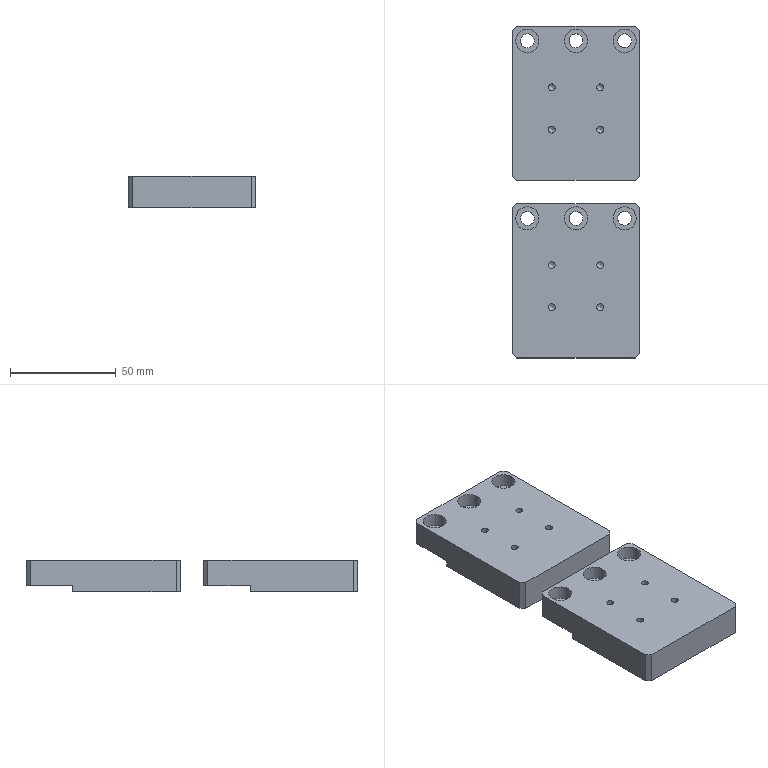Part | 2 solids | 58 faces | box 60 x 157 x 15 mm | volume 117752 mm3 | plane 30 | cylinder 20 | cone 8 | commonest cylinder face diameters 3.3 x8 6.6 x6 11 x6
STEP:
#1=CARTESIAN_POINT('',(-30.,14.5,-7.5));
#2=VERTEX_POINT('',#1);
#3=CARTESIAN_POINT('',(-30.,14.5,-4.5));
#4=VERTEX_POINT('',#3);
#5=CARTESIAN_POINT('',(-30.,14.5,-7.5));
#6=DIRECTION('',(0.,0.,1.));
#7=VECTOR('',#6,1000.);
#8=LINE('',#5,#7);
#9=EDGE_CURVE('',#2,#4,#8,.T.);
#10=ORIENTED_EDGE('',*,*,#9,.T.);
#11=CARTESIAN_POINT('',(30.,14.5,-4.5));
#12=VERTEX_POINT('',#11);
#13=CARTESIAN_POINT('',(30.,14.5,-4.5));
#14=DIRECTION('',(-1.,0.,0.));
#15=VECTOR('',#14,1000.);
#16=LINE('',#13,#15);
#17=EDGE_CURVE('',#12,#4,#16,.T.);
#18=ORIENTED_EDGE('',*,*,#17,.F.);
#19=CARTESIAN_POINT('',(30.,14.5,-7.5));
#20=VERTEX_POINT('',#19);
#21=CARTESIAN_POINT('',(30.,14.5,-7.5));
#22=DIRECTION('',(0.,0.,1.));
#23=VECTOR('',#22,1000.);
#24=LINE('',#21,#23);
#25=EDGE_CURVE('',#20,#12,#24,.T.);
#26=ORIENTED_EDGE('',*,*,#25,.F.);
#27=CARTESIAN_POINT('',(30.,14.5,-7.5));
#28=DIRECTION('',(-1.,0.,0.));
#29=VECTOR('',#28,1000.);
#30=LINE('',#27,#29);
#31=EDGE_CURVE('',#20,#2,#30,.T.);
#32=ORIENTED_EDGE('',*,*,#31,.T.);
#33=EDGE_LOOP('',(#10,#18,#26,#32));
#34=FACE_BOUND('',#33,.T.);
#35=CARTESIAN_POINT('',(30.,14.5,-7.5));
#36=DIRECTION('',(0.,-1.,0.));
#37=DIRECTION('',(1.,0.,0.));
#38=AXIS2_PLACEMENT_3D('',#35,#36,#37);
#39=PLANE('',#38);
#40=ADVANCED_FACE('',(#34),#39,.F.);
#41=CARTESIAN_POINT('',(0.,26.2,-4.5));
#42=VERTEX_POINT('',#41);
#43=CARTESIAN_POINT('',(0.,29.5,-4.5));
#44=DIRECTION('',(0.,0.,-1.));
#45=DIRECTION('',(0.,-1.,0.));
#46=AXIS2_PLACEMENT_3D('',#43,#44,#45);
#47=CIRCLE('',#46,3.3);
#48=EDGE_CURVE('',#42,#42,#47,.T.);
#49=ORIENTED_EDGE('',*,*,#48,.F.);
#50=EDGE_LOOP('',(#49));
#51=FACE_BOUND('',#50,.T.);
#52=CARTESIAN_POINT('',(23.,26.2,-4.5));
#53=VERTEX_POINT('',#52);
#54=CARTESIAN_POINT('',(23.,29.5,-4.5));
#55=DIRECTION('',(0.,0.,-1.));
#56=DIRECTION('',(0.,-1.,0.));
#57=AXIS2_PLACEMENT_3D('',#54,#55,#56);
#58=CIRCLE('',#57,3.3);
#59=EDGE_CURVE('',#53,#53,#58,.T.);
#60=ORIENTED_EDGE('',*,*,#59,.F.);
#61=EDGE_LOOP('',(#60));
#62=FACE_BOUND('',#61,.T.);
#63=CARTESIAN_POINT('',(-23.,26.2,-4.5));
#64=VERTEX_POINT('',#63);
#65=CARTESIAN_POINT('',(-23.,29.5,-4.5));
#66=DIRECTION('',(0.,0.,-1.));
#67=DIRECTION('',(0.,-1.,0.));
#68=AXIS2_PLACEMENT_3D('',#65,#66,#67);
#69=CIRCLE('',#68,3.3);
#70=EDGE_CURVE('',#64,#64,#69,.T.);
#71=ORIENTED_EDGE('',*,*,#70,.F.);
#72=EDGE_LOOP('',(#71));
#73=FACE_BOUND('',#72,.T.);
#74=CARTESIAN_POINT('',(28.,36.5,-4.5));
#75=VERTEX_POINT('',#74);
#76=CARTESIAN_POINT('',(30.,34.5,-4.5));
#77=VERTEX_POINT('',#76);
#78=CARTESIAN_POINT('',(28.,36.5,-4.5));
#79=DIRECTION('',(0.7071,-0.7071,0.));
#80=VECTOR('',#79,1000.);
#81=LINE('',#78,#80);
#82=EDGE_CURVE('',#75,#77,#81,.T.);
#83=ORIENTED_EDGE('',*,*,#82,.T.);
#84=CARTESIAN_POINT('',(30.,36.5,-4.5));
#85=DIRECTION('',(0.,1.,0.));
#86=VECTOR('',#85,1000.);
#87=LINE('',#84,#86);
#88=EDGE_CURVE('',#12,#77,#87,.T.);
#89=ORIENTED_EDGE('',*,*,#88,.F.);
#90=ORIENTED_EDGE('',*,*,#17,.T.);
#91=CARTESIAN_POINT('',(-30.,34.5,-4.5));
#92=VERTEX_POINT('',#91);
#93=CARTESIAN_POINT('',(-30.,36.5,-4.5));
#94=DIRECTION('',(0.,1.,0.));
#95=VECTOR('',#94,1000.);
#96=LINE('',#93,#95);
#97=EDGE_CURVE('',#4,#92,#96,.T.);
#98=ORIENTED_EDGE('',*,*,#97,.T.);
#99=CARTESIAN_POINT('',(-28.,36.5,-4.5));
#100=VERTEX_POINT('',#99);
#101=CARTESIAN_POINT('',(-30.,34.5,-4.5));
#102=DIRECTION('',(0.7071,0.7071,0.));
#103=VECTOR('',#102,1000.);
#104=LINE('',#101,#103);
#105=EDGE_CURVE('',#92,#100,#104,.T.);
#106=ORIENTED_EDGE('',*,*,#105,.T.);
#107=CARTESIAN_POINT('',(30.,36.5,-4.5));
#108=DIRECTION('',(-1.,0.,0.));
#109=VECTOR('',#108,1000.);
#110=LINE('',#107,#109);
#111=EDGE_CURVE('',#75,#100,#110,.T.);
#112=ORIENTED_EDGE('',*,*,#111,.F.);
#113=EDGE_LOOP('',(#83,#89,#90,#98,#106,#112));
#114=FACE_BOUND('',#113,.T.);
#115=CARTESIAN_POINT('',(30.,36.5,-4.5));
#116=DIRECTION('',(0.,0.,1.));
#117=DIRECTION('',(0.,-1.,0.));
#118=AXIS2_PLACEMENT_3D('',#115,#116,#117);
#119=PLANE('',#118);
#120=ADVANCED_FACE('',(#51,#62,#73,#114),#119,.F.);
#121=CARTESIAN_POINT('',(28.5,29.5,1.1));
#122=VERTEX_POINT('',#121);
#123=CARTESIAN_POINT('',(23.,29.5,1.1));
#124=DIRECTION('',(0.,0.,1.));
#125=DIRECTION('',(1.,0.,0.));
#126=AXIS2_PLACEMENT_3D('',#123,#124,#125);
#127=CIRCLE('',#126,5.5);
#128=EDGE_CURVE('',#122,#122,#127,.T.);
#129=ORIENTED_EDGE('',*,*,#128,.T.);
#130=EDGE_LOOP('',(#129));
#131=FACE_BOUND('',#130,.T.);
#132=CARTESIAN_POINT('',(26.3,29.5,1.1));
#133=VERTEX_POINT('',#132);
#134=CARTESIAN_POINT('',(23.,29.5,1.1));
#135=DIRECTION('',(0.,0.,1.));
#136=DIRECTION('',(1.,0.,0.));
#137=AXIS2_PLACEMENT_3D('',#134,#135,#136);
#138=CIRCLE('',#137,3.3);
#139=EDGE_CURVE('',#133,#133,#138,.T.);
#140=ORIENTED_EDGE('',*,*,#139,.F.);
#141=EDGE_LOOP('',(#140));
#142=FACE_BOUND('',#141,.T.);
#143=CARTESIAN_POINT('',(26.3,29.5,1.1));
#144=DIRECTION('',(0.,0.,-1.));
#145=DIRECTION('',(-1.,0.,0.));
#146=AXIS2_PLACEMENT_3D('',#143,#144,#145);
#147=PLANE('',#146);
#148=ADVANCED_FACE('',(#131,#142),#147,.F.);
#149=CARTESIAN_POINT('',(-28.5,29.5,1.1));
#150=VERTEX_POINT('',#149);
#151=CARTESIAN_POINT('',(-23.,29.5,1.1));
#152=DIRECTION('',(0.,0.,1.));
#153=DIRECTION('',(-1.,0.,0.));
#154=AXIS2_PLACEMENT_3D('',#151,#152,#153);
#155=CIRCLE('',#154,5.5);
#156=EDGE_CURVE('',#150,#150,#155,.T.);
#157=ORIENTED_EDGE('',*,*,#156,.T.);
#158=EDGE_LOOP('',(#157));
#159=FACE_BOUND('',#158,.T.);
#160=CARTESIAN_POINT('',(-26.3,29.5,1.1));
#161=VERTEX_POINT('',#160);
#162=CARTESIAN_POINT('',(-23.,29.5,1.1));
#163=DIRECTION('',(0.,0.,1.));
#164=DIRECTION('',(-1.,0.,0.));
#165=AXIS2_PLACEMENT_3D('',#162,#163,#164);
#166=CIRCLE('',#165,3.3);
#167=EDGE_CURVE('',#161,#161,#166,.T.);
#168=ORIENTED_EDGE('',*,*,#167,.F.);
#169=EDGE_LOOP('',(#168));
#170=FACE_BOUND('',#169,.T.);
#171=CARTESIAN_POINT('',(26.3,29.5,1.1));
#172=DIRECTION('',(0.,0.,-1.));
#173=DIRECTION('',(-1.,0.,0.));
#174=AXIS2_PLACEMENT_3D('',#171,#172,#173);
#175=PLANE('',#174);
#176=ADVANCED_FACE('',(#159,#170),#175,.F.);
#177=CARTESIAN_POINT('',(-5.5,29.5,1.1));
#178=VERTEX_POINT('',#177);
#179=CARTESIAN_POINT('',(0.,29.5,1.1));
#180=DIRECTION('',(0.,0.,1.));
#181=DIRECTION('',(-1.,0.,0.));
#182=AXIS2_PLACEMENT_3D('',#179,#180,#181);
#183=CIRCLE('',#182,5.5);
#184=EDGE_CURVE('',#178,#178,#183,.T.);
#185=ORIENTED_EDGE('',*,*,#184,.T.);
#186=EDGE_LOOP('',(#185));
#187=FACE_BOUND('',#186,.T.);
#188=CARTESIAN_POINT('',(-3.3,29.5,1.1));
#189=VERTEX_POINT('',#188);
#190=CARTESIAN_POINT('',(0.,29.5,1.1));
#191=DIRECTION('',(0.,0.,1.));
#192=DIRECTION('',(-1.,0.,0.));
#193=AXIS2_PLACEMENT_3D('',#190,#191,#192);
#194=CIRCLE('',#193,3.3);
#195=EDGE_CURVE('',#189,#189,#194,.T.);
#196=ORIENTED_EDGE('',*,*,#195,.F.);
#197=EDGE_LOOP('',(#196));
#198=FACE_BOUND('',#197,.T.);
#199=CARTESIAN_POINT('',(26.3,29.5,1.1));
#200=DIRECTION('',(0.,0.,-1.));
#201=DIRECTION('',(-1.,0.,0.));
#202=AXIS2_PLACEMENT_3D('',#199,#200,#201);
#203=PLANE('',#202);
#204=ADVANCED_FACE('',(#187,#198),#203,.F.);
#205=ORIENTED_EDGE('',*,*,#105,.F.);
#206=CARTESIAN_POINT('',(-30.,34.5,7.5));
#207=VERTEX_POINT('',#206);
#208=CARTESIAN_POINT('',(-30.,34.5,7.5));
#209=DIRECTION('',(0.,0.,-1.));
#210=VECTOR('',#209,1000.);
#211=LINE('',#208,#210);
#212=EDGE_CURVE('',#207,#92,#211,.T.);
#213=ORIENTED_EDGE('',*,*,#212,.F.);
#214=CARTESIAN_POINT('',(-28.,36.5,7.5));
#215=VERTEX_POINT('',#214);
#216=CARTESIAN_POINT('',(-32.25,32.25,7.5));
#217=DIRECTION('',(-0.7071,-0.7071,0.));
#218=VECTOR('',#217,1000.);
#219=LINE('',#216,#218);
#220=EDGE_CURVE('',#215,#207,#219,.T.);
#221=ORIENTED_EDGE('',*,*,#220,.F.);
#222=CARTESIAN_POINT('',(-28.,36.5,7.5));
#223=DIRECTION('',(0.,0.,1.));
#224=VECTOR('',#223,1000.);
#225=LINE('',#222,#224);
#226=EDGE_CURVE('',#100,#215,#225,.T.);
#227=ORIENTED_EDGE('',*,*,#226,.F.);
#228=EDGE_LOOP('',(#205,#213,#221,#227));
#229=FACE_BOUND('',#228,.T.);
#230=CARTESIAN_POINT('',(-30.,34.5,7.5));
#231=DIRECTION('',(0.7071,-0.7071,0.));
#232=DIRECTION('',(0.,0.,-1.));
#233=AXIS2_PLACEMENT_3D('',#230,#231,#232);
#234=PLANE('',#233);
#235=ADVANCED_FACE('',(#229),#234,.F.);
#236=ORIENTED_EDGE('',*,*,#82,.F.);
#237=CARTESIAN_POINT('',(28.,36.5,7.5));
#238=VERTEX_POINT('',#237);
#239=CARTESIAN_POINT('',(28.,36.5,7.5));
#240=DIRECTION('',(0.,0.,-1.));
#241=VECTOR('',#240,1000.);
#242=LINE('',#239,#241);
#243=EDGE_CURVE('',#238,#75,#242,.T.);
#244=ORIENTED_EDGE('',*,*,#243,.F.);
#245=CARTESIAN_POINT('',(30.,34.5,7.5));
#246=VERTEX_POINT('',#245);
#247=CARTESIAN_POINT('',(32.25,32.25,7.5));
#248=DIRECTION('',(-0.7071,0.7071,0.));
#249=VECTOR('',#248,1000.);
#250=LINE('',#247,#249);
#251=EDGE_CURVE('',#246,#238,#250,.T.);
#252=ORIENTED_EDGE('',*,*,#251,.F.);
#253=CARTESIAN_POINT('',(30.,34.5,7.5));
#254=DIRECTION('',(0.,0.,1.));
#255=VECTOR('',#254,1000.);
#256=LINE('',#253,#255);
#257=EDGE_CURVE('',#77,#246,#256,.T.);
#258=ORIENTED_EDGE('',*,*,#257,.F.);
#259=EDGE_LOOP('',(#236,#244,#252,#258));
#260=FACE_BOUND('',#259,.T.);
#261=CARTESIAN_POINT('',(28.,36.5,7.5));
#262=DIRECTION('',(-0.7071,-0.7071,0.));
#263=DIRECTION('',(0.,0.,-1.));
#264=AXIS2_PLACEMENT_3D('',#261,#262,#263);
#265=PLANE('',#264);
#266=ADVANCED_FACE('',(#260),#265,.F.);
#267=CARTESIAN_POINT('',(28.,-36.5,7.5));
#268=VERTEX_POINT('',#267);
#269=CARTESIAN_POINT('',(30.,-34.5,7.5));
#270=VERTEX_POINT('',#269);
#271=CARTESIAN_POINT('',(32.25,-32.25,7.5));
#272=DIRECTION('',(0.7071,0.7071,0.));
#273=VECTOR('',#272,1000.);
#274=LINE('',#271,#273);
#275=EDGE_CURVE('',#268,#270,#274,.T.);
#276=ORIENTED_EDGE('',*,*,#275,.F.);
#277=CARTESIAN_POINT('',(28.,-36.5,-7.5));
#278=VERTEX_POINT('',#277);
#279=CARTESIAN_POINT('',(28.,-36.5,7.5));
#280=DIRECTION('',(0.,0.,1.));
#281=VECTOR('',#280,1000.);
#282=LINE('',#279,#281);
#283=EDGE_CURVE('',#278,#268,#282,.T.);
#284=ORIENTED_EDGE('',*,*,#283,.F.);
#285=CARTESIAN_POINT('',(30.,-34.5,-7.5));
#286=VERTEX_POINT('',#285);
#287=CARTESIAN_POINT('',(30.,-34.5,-7.5));
#288=DIRECTION('',(-0.7071,-0.7071,0.));
#289=VECTOR('',#288,1000.);
#290=LINE('',#287,#289);
#291=EDGE_CURVE('',#286,#278,#290,.T.);
#292=ORIENTED_EDGE('',*,*,#291,.F.);
#293=CARTESIAN_POINT('',(30.,-34.5,7.5));
#294=DIRECTION('',(0.,0.,-1.));
#295=VECTOR('',#294,1000.);
#296=LINE('',#293,#295);
#297=EDGE_CURVE('',#270,#286,#296,.T.);
#298=ORIENTED_EDGE('',*,*,#297,.F.);
#299=EDGE_LOOP('',(#276,#284,#292,#298));
#300=FACE_BOUND('',#299,.T.);
#301=CARTESIAN_POINT('',(30.,-34.5,7.5));
#302=DIRECTION('',(-0.7071,0.7071,0.));
#303=DIRECTION('',(0.,0.,-1.));
#304=AXIS2_PLACEMENT_3D('',#301,#302,#303);
#305=PLANE('',#304);
#306=ADVANCED_FACE('',(#300),#305,.F.);
#307=CARTESIAN_POINT('',(-30.,-34.5,7.5));
#308=VERTEX_POINT('',#307);
#309=CARTESIAN_POINT('',(-28.,-36.5,7.5));
#310=VERTEX_POINT('',#309);
#311=CARTESIAN_POINT('',(-32.25,-32.25,7.5));
#312=DIRECTION('',(0.7071,-0.7071,0.));
#313=VECTOR('',#312,1000.);
#314=LINE('',#311,#313);
#315=EDGE_CURVE('',#308,#310,#314,.T.);
#316=ORIENTED_EDGE('',*,*,#315,.F.);
#317=CARTESIAN_POINT('',(-30.,-34.5,-7.5));
#318=VERTEX_POINT('',#317);
#319=CARTESIAN_POINT('',(-30.,-34.5,7.5));
#320=DIRECTION('',(0.,0.,1.));
#321=VECTOR('',#320,1000.);
#322=LINE('',#319,#321);
#323=EDGE_CURVE('',#318,#308,#322,.T.);
#324=ORIENTED_EDGE('',*,*,#323,.F.);
#325=CARTESIAN_POINT('',(-28.,-36.5,-7.5));
#326=VERTEX_POINT('',#325);
#327=CARTESIAN_POINT('',(-28.,-36.5,-7.5));
#328=DIRECTION('',(-0.7071,0.7071,0.));
#329=VECTOR('',#328,1000.);
#330=LINE('',#327,#329);
#331=EDGE_CURVE('',#326,#318,#330,.T.);
#332=ORIENTED_EDGE('',*,*,#331,.F.);
#333=CARTESIAN_POINT('',(-28.,-36.5,7.5));
#334=DIRECTION('',(0.,0.,-1.));
#335=VECTOR('',#334,1000.);
#336=LINE('',#333,#335);
#337=EDGE_CURVE('',#310,#326,#336,.T.);
#338=ORIENTED_EDGE('',*,*,#337,.F.);
#339=EDGE_LOOP('',(#316,#324,#332,#338));
#340=FACE_BOUND('',#339,.T.);
#341=CARTESIAN_POINT('',(-28.,-36.5,7.5));
#342=DIRECTION('',(0.7071,0.7071,0.));
#343=DIRECTION('',(0.,0.,-1.));
#344=AXIS2_PLACEMENT_3D('',#341,#342,#343);
#345=PLANE('',#344);
#346=ADVANCED_FACE('',(#340),#345,.F.);
#347=CARTESIAN_POINT('',(-30.,36.5,-7.5));
#348=DIRECTION('',(0.,-1.,0.));
#349=VECTOR('',#348,1000.);
#350=LINE('',#347,#349);
#351=EDGE_CURVE('',#2,#318,#350,.T.);
#352=ORIENTED_EDGE('',*,*,#351,.F.);
#353=ORIENTED_EDGE('',*,*,#31,.F.);
#354=CARTESIAN_POINT('',(30.,36.5,-7.5));
#355=DIRECTION('',(0.,1.,0.));
#356=VECTOR('',#355,1000.);
#357=LINE('',#354,#356);
#358=EDGE_CURVE('',#286,#20,#357,.T.);
#359=ORIENTED_EDGE('',*,*,#358,.F.);
#360=ORIENTED_EDGE('',*,*,#291,.T.);
#361=CARTESIAN_POINT('',(-30.,-36.5,-7.5));
#362=DIRECTION('',(1.,0.,0.));
#363=VECTOR('',#362,1000.);
#364=LINE('',#361,#363);
#365=EDGE_CURVE('',#326,#278,#364,.T.);
#366=ORIENTED_EDGE('',*,*,#365,.F.);
#367=ORIENTED_EDGE('',*,*,#331,.T.);
#368=EDGE_LOOP('',(#352,#353,#359,#360,#366,#367));
#369=FACE_BOUND('',#368,.T.);
#370=CARTESIAN_POINT('',(0.,0.,-7.5));
#371=DIRECTION('',(0.,0.,1.));
#372=DIRECTION('',(1.,0.,0.));
#373=AXIS2_PLACEMENT_3D('',#370,#371,#372);
#374=PLANE('',#373);
#375=ADVANCED_FACE('',(#369),#374,.F.);
#376=CARTESIAN_POINT('',(-30.,36.5,7.5));
#377=DIRECTION('',(0.,-1.,0.));
#378=VECTOR('',#377,1000.);
#379=LINE('',#376,#378);
#380=EDGE_CURVE('',#207,#308,#379,.T.);
#381=ORIENTED_EDGE('',*,*,#380,.T.);
#382=ORIENTED_EDGE('',*,*,#315,.T.);
#383=CARTESIAN_POINT('',(-30.,-36.5,7.5));
#384=DIRECTION('',(1.,0.,0.));
#385=VECTOR('',#384,1000.);
#386=LINE('',#383,#385);
#387=EDGE_CURVE('',#310,#268,#386,.T.);
#388=ORIENTED_EDGE('',*,*,#387,.T.);
#389=ORIENTED_EDGE('',*,*,#275,.T.);
#390=CARTESIAN_POINT('',(30.,36.5,7.5));
#391=DIRECTION('',(0.,1.,0.));
#392=VECTOR('',#391,1000.);
#393=LINE('',#390,#392);
#394=EDGE_CURVE('',#270,#246,#393,.T.);
#395=ORIENTED_EDGE('',*,*,#394,.T.);
#396=ORIENTED_EDGE('',*,*,#251,.T.);
#397=CARTESIAN_POINT('',(-30.,36.5,7.5));
#398=DIRECTION('',(-1.,0.,0.));
#399=VECTOR('',#398,1000.);
#400=LINE('',#397,#399);
#401=EDGE_CURVE('',#238,#215,#400,.T.);
#402=ORIENTED_EDGE('',*,*,#401,.T.);
#403=ORIENTED_EDGE('',*,*,#220,.T.);
#404=EDGE_LOOP('',(#381,#382,#388,#389,#395,#396,#402,#403));
#405=FACE_BOUND('',#404,.T.);
#406=CARTESIAN_POINT('',(13.15,7.5,7.5));
#407=VERTEX_POINT('',#406);
#408=CARTESIAN_POINT('',(11.5,7.5,7.5));
#409=DIRECTION('',(0.,0.,1.));
#410=DIRECTION('',(1.,0.,0.));
#411=AXIS2_PLACEMENT_3D('',#408,#409,#410);
#412=CIRCLE('',#411,1.65);
#413=EDGE_CURVE('',#407,#407,#412,.T.);
#414=ORIENTED_EDGE('',*,*,#413,.F.);
#415=EDGE_LOOP('',(#414));
#416=FACE_BOUND('',#415,.T.);
#417=CARTESIAN_POINT('',(13.15,-12.5,7.5));
#418=VERTEX_POINT('',#417);
#419=CARTESIAN_POINT('',(11.5,-12.5,7.5));
#420=DIRECTION('',(0.,0.,1.));
#421=DIRECTION('',(1.,0.,0.));
#422=AXIS2_PLACEMENT_3D('',#419,#420,#421);
#423=CIRCLE('',#422,1.65);
#424=EDGE_CURVE('',#418,#418,#423,.T.);
#425=ORIENTED_EDGE('',*,*,#424,.F.);
#426=EDGE_LOOP('',(#425));
#427=FACE_BOUND('',#426,.T.);
#428=CARTESIAN_POINT('',(-9.85,-12.5,7.5));
#429=VERTEX_POINT('',#428);
#430=CARTESIAN_POINT('',(-11.5,-12.5,7.5));
#431=DIRECTION('',(0.,0.,1.));
#432=DIRECTION('',(1.,0.,0.));
#433=AXIS2_PLACEMENT_3D('',#430,#431,#432);
#434=CIRCLE('',#433,1.65);
#435=EDGE_CURVE('',#429,#429,#434,.T.);
#436=ORIENTED_EDGE('',*,*,#435,.F.);
#437=EDGE_LOOP('',(#436));
#438=FACE_BOUND('',#437,.T.);
#439=CARTESIAN_POINT('',(-9.85,7.5,7.5));
#440=VERTEX_POINT('',#439);
#441=CARTESIAN_POINT('',(-11.5,7.5,7.5));
#442=DIRECTION('',(0.,0.,1.));
#443=DIRECTION('',(1.,0.,0.));
#444=AXIS2_PLACEMENT_3D('',#441,#442,#443);
#445=CIRCLE('',#444,1.65);
#446=EDGE_CURVE('',#440,#440,#445,.T.);
#447=ORIENTED_EDGE('',*,*,#446,.F.);
#448=EDGE_LOOP('',(#447));
#449=FACE_BOUND('',#448,.T.);
#450=CARTESIAN_POINT('',(5.5,29.5,7.5));
#451=VERTEX_POINT('',#450);
#452=CARTESIAN_POINT('',(0.,29.5,7.5));
#453=DIRECTION('',(0.,0.,1.));
#454=DIRECTION('',(1.,0.,0.));
#455=AXIS2_PLACEMENT_3D('',#452,#453,#454);
#456=CIRCLE('',#455,5.5);
#457=EDGE_CURVE('',#451,#451,#456,.T.);
#458=ORIENTED_EDGE('',*,*,#457,.F.);
#459=EDGE_LOOP('',(#458));
#460=FACE_BOUND('',#459,.T.);
#461=CARTESIAN_POINT('',(-17.5,29.5,7.5));
#462=VERTEX_POINT('',#461);
#463=CARTESIAN_POINT('',(-23.,29.5,7.5));
#464=DIRECTION('',(0.,0.,1.));
#465=DIRECTION('',(1.,0.,0.));
#466=AXIS2_PLACEMENT_3D('',#463,#464,#465);
#467=CIRCLE('',#466,5.5);
#468=EDGE_CURVE('',#462,#462,#467,.T.);
#469=ORIENTED_EDGE('',*,*,#468,.F.);
#470=EDGE_LOOP('',(#469));
#471=FACE_BOUND('',#470,.T.);
#472=CARTESIAN_POINT('',(28.5,29.5,7.5));
#473=VERTEX_POINT('',#472);
#474=CARTESIAN_POINT('',(23.,29.5,7.5));
#475=DIRECTION('',(0.,0.,1.));
#476=DIRECTION('',(1.,0.,0.));
#477=AXIS2_PLACEMENT_3D('',#474,#475,#476);
#478=CIRCLE('',#477,5.5);
#479=EDGE_CURVE('',#473,#473,#478,.T.);
#480=ORIENTED_EDGE('',*,*,#479,.F.);
#481=EDGE_LOOP('',(#480));
#482=FACE_BOUND('',#481,.T.);
#483=CARTESIAN_POINT('',(0.,0.,7.5));
#484=DIRECTION('',(0.,0.,1.));
#485=DIRECTION('',(1.,0.,0.));
#486=AXIS2_PLACEMENT_3D('',#483,#484,#485);
#487=PLANE('',#486);
#488=ADVANCED_FACE('',(#405,#416,#427,#438,#449,#460,#471,#482),#487,.T.);
#489=ORIENTED_EDGE('',*,*,#387,.F.);
#490=ORIENTED_EDGE('',*,*,#337,.T.);
#491=ORIENTED_EDGE('',*,*,#365,.T.);
#492=ORIENTED_EDGE('',*,*,#283,.T.);
#493=EDGE_LOOP('',(#489,#490,#491,#492));
#494=FACE_BOUND('',#493,.T.);
#495=CARTESIAN_POINT('',(-30.,-36.5,7.5));
#496=DIRECTION('',(0.,1.,0.));
#497=DIRECTION('',(0.,0.,1.));
#498=AXIS2_PLACEMENT_3D('',#495,#496,#497);
#499=PLANE('',#498);
#500=ADVANCED_FACE('',(#494),#499,.F.);
#501=ORIENTED_EDGE('',*,*,#212,.T.);
#502=ORIENTED_EDGE('',*,*,#97,.F.);
#503=ORIENTED_EDGE('',*,*,#9,.F.);
#504=ORIENTED_EDGE('',*,*,#351,.T.);
#505=ORIENTED_EDGE('',*,*,#323,.T.);
#506=ORIENTED_EDGE('',*,*,#380,.F.);
#507=EDGE_LOOP('',(#501,#502,#503,#504,#505,#506));
#508=FACE_BOUND('',#507,.T.);
#509=CARTESIAN_POINT('',(-30.,36.5,7.5));
#510=DIRECTION('',(1.,0.,0.));
#511=DIRECTION('',(0.,1.,0.));
#512=AXIS2_PLACEMENT_3D('',#509,#510,#511);
#513=PLANE('',#512);
#514=ADVANCED_FACE('',(#508),#513,.F.);
#515=ORIENTED_EDGE('',*,*,#243,.T.);
#516=ORIENTED_EDGE('',*,*,#111,.T.);
#517=ORIENTED_EDGE('',*,*,#226,.T.);
#518=ORIENTED_EDGE('',*,*,#401,.F.);
#519=EDGE_LOOP('',(#515,#516,#517,#518));
#520=FACE_BOUND('',#519,.T.);
#521=CARTESIAN_POINT('',(-30.,36.5,7.5));
#522=DIRECTION('',(0.,-1.,0.));
#523=DIRECTION('',(0.,0.,-1.));
#524=AXIS2_PLACEMENT_3D('',#521,#522,#523);
#525=PLANE('',#524);
#526=ADVANCED_FACE('',(#520),#525,.F.);
#527=ORIENTED_EDGE('',*,*,#25,.T.);
#528=ORIENTED_EDGE('',*,*,#88,.T.);
#529=ORIENTED_EDGE('',*,*,#257,.T.);
#530=ORIENTED_EDGE('',*,*,#394,.F.);
#531=ORIENTED_EDGE('',*,*,#297,.T.);
#532=ORIENTED_EDGE('',*,*,#358,.T.);
#533=EDGE_LOOP('',(#527,#528,#529,#530,#531,#532));
#534=FACE_BOUND('',#533,.T.);
#535=CARTESIAN_POINT('',(30.,36.5,7.5));
#536=DIRECTION('',(-1.,0.,0.));
#537=DIRECTION('',(0.,-1.,0.));
#538=AXIS2_PLACEMENT_3D('',#535,#536,#537);
#539=PLANE('',#538);
#540=ADVANCED_FACE('',(#534),#539,.F.);
#541=CARTESIAN_POINT('',(13.15,7.5,-2.6));
#542=VERTEX_POINT('',#541);
#543=CARTESIAN_POINT('',(11.5,7.5,-2.6));
#544=DIRECTION('',(0.,0.,1.));
#545=DIRECTION('',(1.,0.,0.));
#546=AXIS2_PLACEMENT_3D('',#543,#544,#545);
#547=CIRCLE('',#546,1.65);
#548=EDGE_CURVE('',#542,#542,#547,.T.);
#549=ORIENTED_EDGE('',*,*,#548,.T.);
#550=EDGE_LOOP('',(#549));
#551=FACE_BOUND('',#550,.T.);
#552=CARTESIAN_POINT('',(11.5,7.5,-3.591));
#553=VERTEX_POINT('',#552);
#554=VERTEX_LOOP('',#553);
#555=FACE_BOUND('',#554,.T.);
#556=CARTESIAN_POINT('',(11.5,7.5,-2.6));
#557=DIRECTION('',(0.,0.,1.));
#558=DIRECTION('',(1.,0.,0.));
#559=AXIS2_PLACEMENT_3D('',#556,#557,#558);
#560=CONICAL_SURFACE('',#559,1.65,1.03);
#561=ADVANCED_FACE('',(#551,#555),#560,.F.);
#562=ORIENTED_EDGE('',*,*,#548,.F.);
#563=EDGE_LOOP('',(#562));
#564=FACE_BOUND('',#563,.T.);
#565=ORIENTED_EDGE('',*,*,#413,.T.);
#566=EDGE_LOOP('',(#565));
#567=FACE_BOUND('',#566,.T.);
#568=CARTESIAN_POINT('',(11.5,7.5,7.5));
#569=DIRECTION('',(0.,0.,1.));
#570=DIRECTION('',(1.,0.,0.));
#571=AXIS2_PLACEMENT_3D('',#568,#569,#570);
#572=CYLINDRICAL_SURFACE('',#571,1.65);
#573=ADVANCED_FACE('',(#564,#567),#572,.F.);
#574=CARTESIAN_POINT('',(13.15,-12.5,-2.6));
#575=VERTEX_POINT('',#574);
#576=CARTESIAN_POINT('',(11.5,-12.5,-2.6));
#577=DIRECTION('',(0.,0.,1.));
#578=DIRECTION('',(1.,0.,0.));
#579=AXIS2_PLACEMENT_3D('',#576,#577,#578);
#580=CIRCLE('',#579,1.65);
#581=EDGE_CURVE('',#575,#575,#580,.T.);
#582=ORIENTED_EDGE('',*,*,#581,.T.);
#583=EDGE_LOOP('',(#582));
#584=FACE_BOUND('',#583,.T.);
#585=CARTESIAN_POINT('',(11.5,-12.5,-3.591));
#586=VERTEX_POINT('',#585);
#587=VERTEX_LOOP('',#586);
#588=FACE_BOUND('',#587,.T.);
#589=CARTESIAN_POINT('',(11.5,-12.5,-2.6));
#590=DIRECTION('',(0.,0.,1.));
#591=DIRECTION('',(1.,0.,0.));
#592=AXIS2_PLACEMENT_3D('',#589,#590,#591);
#593=CONICAL_SURFACE('',#592,1.65,1.03);
#594=ADVANCED_FACE('',(#584,#588),#593,.F.);
#595=ORIENTED_EDGE('',*,*,#581,.F.);
#596=EDGE_LOOP('',(#595));
#597=FACE_BOUND('',#596,.T.);
#598=ORIENTED_EDGE('',*,*,#424,.T.);
#599=EDGE_LOOP('',(#598));
#600=FACE_BOUND('',#599,.T.);
#601=CARTESIAN_POINT('',(11.5,-12.5,7.5));
#602=DIRECTION('',(0.,0.,1.));
#603=DIRECTION('',(1.,0.,0.));
#604=AXIS2_PLACEMENT_3D('',#601,#602,#603);
#605=CYLINDRICAL_SURFACE('',#604,1.65);
#606=ADVANCED_FACE('',(#597,#600),#605,.F.);
#607=CARTESIAN_POINT('',(-9.85,-12.5,-2.6));
#608=VERTEX_POINT('',#607);
#609=CARTESIAN_POINT('',(-11.5,-12.5,-2.6));
#610=DIRECTION('',(0.,0.,1.));
#611=DIRECTION('',(1.,0.,0.));
#612=AXIS2_PLACEMENT_3D('',#609,#610,#611);
#613=CIRCLE('',#612,1.65);
#614=EDGE_CURVE('',#608,#608,#613,.T.);
#615=ORIENTED_EDGE('',*,*,#614,.T.);
#616=EDGE_LOOP('',(#615));
#617=FACE_BOUND('',#616,.T.);
#618=CARTESIAN_POINT('',(-11.5,-12.5,-3.591));
#619=VERTEX_POINT('',#618);
#620=VERTEX_LOOP('',#619);
#621=FACE_BOUND('',#620,.T.);
#622=CARTESIAN_POINT('',(-11.5,-12.5,-2.6));
#623=DIRECTION('',(0.,0.,1.));
#624=DIRECTION('',(1.,0.,0.));
#625=AXIS2_PLACEMENT_3D('',#622,#623,#624);
#626=CONICAL_SURFACE('',#625,1.65,1.03);
#627=ADVANCED_FACE('',(#617,#621),#626,.F.);
#628=ORIENTED_EDGE('',*,*,#614,.F.);
#629=EDGE_LOOP('',(#628));
#630=FACE_BOUND('',#629,.T.);
#631=ORIENTED_EDGE('',*,*,#435,.T.);
#632=EDGE_LOOP('',(#631));
#633=FACE_BOUND('',#632,.T.);
#634=CARTESIAN_POINT('',(-11.5,-12.5,7.5));
#635=DIRECTION('',(0.,0.,1.));
#636=DIRECTION('',(1.,0.,0.));
#637=AXIS2_PLACEMENT_3D('',#634,#635,#636);
#638=CYLINDRICAL_SURFACE('',#637,1.65);
#639=ADVANCED_FACE('',(#630,#633),#638,.F.);
#640=CARTESIAN_POINT('',(-9.85,7.5,-2.6));
#641=VERTEX_POINT('',#640);
#642=CARTESIAN_POINT('',(-11.5,7.5,-2.6));
#643=DIRECTION('',(0.,0.,1.));
#644=DIRECTION('',(1.,0.,0.));
#645=AXIS2_PLACEMENT_3D('',#642,#643,#644);
#646=CIRCLE('',#645,1.65);
#647=EDGE_CURVE('',#641,#641,#646,.T.);
#648=ORIENTED_EDGE('',*,*,#647,.T.);
#649=EDGE_LOOP('',(#648));
#650=FACE_BOUND('',#649,.T.);
#651=CARTESIAN_POINT('',(-11.5,7.5,-3.591));
#652=VERTEX_POINT('',#651);
#653=VERTEX_LOOP('',#652);
#654=FACE_BOUND('',#653,.T.);
#655=CARTESIAN_POINT('',(-11.5,7.5,-2.6));
#656=DIRECTION('',(0.,0.,1.));
#657=DIRECTION('',(1.,0.,0.));
#658=AXIS2_PLACEMENT_3D('',#655,#656,#657);
#659=CONICAL_SURFACE('',#658,1.65,1.03);
#660=ADVANCED_FACE('',(#650,#654),#659,.F.);
#661=ORIENTED_EDGE('',*,*,#647,.F.);
#662=EDGE_LOOP('',(#661));
#663=FACE_BOUND('',#662,.T.);
#664=ORIENTED_EDGE('',*,*,#446,.T.);
#665=EDGE_LOOP('',(#664));
#666=FACE_BOUND('',#665,.T.);
#667=CARTESIAN_POINT('',(-11.5,7.5,7.5));
#668=DIRECTION('',(0.,0.,1.));
#669=DIRECTION('',(1.,0.,0.));
#670=AXIS2_PLACEMENT_3D('',#667,#668,#669);
#671=CYLINDRICAL_SURFACE('',#670,1.65);
#672=ADVANCED_FACE('',(#663,#666),#671,.F.);
#673=ORIENTED_EDGE('',*,*,#48,.T.);
#674=EDGE_LOOP('',(#673));
#675=FACE_BOUND('',#674,.T.);
#676=ORIENTED_EDGE('',*,*,#195,.T.);
#677=EDGE_LOOP('',(#676));
#678=FACE_BOUND('',#677,.T.);
#679=CARTESIAN_POINT('',(0.,29.5,7.5));
#680=DIRECTION('',(0.,0.,1.));
#681=DIRECTION('',(1.,0.,0.));
#682=AXIS2_PLACEMENT_3D('',#679,#680,#681);
#683=CYLINDRICAL_SURFACE('',#682,3.3);
#684=ADVANCED_FACE('',(#675,#678),#683,.F.);
#685=ORIENTED_EDGE('',*,*,#184,.F.);
#686=EDGE_LOOP('',(#685));
#687=FACE_BOUND('',#686,.T.);
#688=ORIENTED_EDGE('',*,*,#457,.T.);
#689=EDGE_LOOP('',(#688));
#690=FACE_BOUND('',#689,.T.);
#691=CARTESIAN_POINT('',(0.,29.5,7.5));
#692=DIRECTION('',(0.,0.,1.));
#693=DIRECTION('',(1.,0.,0.));
#694=AXIS2_PLACEMENT_3D('',#691,#692,#693);
#695=CYLINDRICAL_SURFACE('',#694,5.5);
#696=ADVANCED_FACE('',(#687,#690),#695,.F.);
#697=ORIENTED_EDGE('',*,*,#70,.T.);
#698=EDGE_LOOP('',(#697));
#699=FACE_BOUND('',#698,.T.);
#700=ORIENTED_EDGE('',*,*,#167,.T.);
#701=EDGE_LOOP('',(#700));
#702=FACE_BOUND('',#701,.T.);
#703=CARTESIAN_POINT('',(-23.,29.5,7.5));
#704=DIRECTION('',(0.,0.,1.));
#705=DIRECTION('',(1.,0.,0.));
#706=AXIS2_PLACEMENT_3D('',#703,#704,#705);
#707=CYLINDRICAL_SURFACE('',#706,3.3);
#708=ADVANCED_FACE('',(#699,#702),#707,.F.);
#709=ORIENTED_EDGE('',*,*,#156,.F.);
#710=EDGE_LOOP('',(#709));
#711=FACE_BOUND('',#710,.T.);
#712=ORIENTED_EDGE('',*,*,#468,.T.);
#713=EDGE_LOOP('',(#712));
#714=FACE_BOUND('',#713,.T.);
#715=CARTESIAN_POINT('',(-23.,29.5,7.5));
#716=DIRECTION('',(0.,0.,1.));
#717=DIRECTION('',(1.,0.,0.));
#718=AXIS2_PLACEMENT_3D('',#715,#716,#717);
#719=CYLINDRICAL_SURFACE('',#718,5.5);
#720=ADVANCED_FACE('',(#711,#714),#719,.F.);
#721=ORIENTED_EDGE('',*,*,#59,.T.);
#722=EDGE_LOOP('',(#721));
#723=FACE_BOUND('',#722,.T.);
#724=ORIENTED_EDGE('',*,*,#139,.T.);
#725=EDGE_LOOP('',(#724));
#726=FACE_BOUND('',#725,.T.);
#727=CARTESIAN_POINT('',(23.,29.5,7.5));
#728=DIRECTION('',(0.,0.,1.));
#729=DIRECTION('',(1.,0.,0.));
#730=AXIS2_PLACEMENT_3D('',#727,#728,#729);
#731=CYLINDRICAL_SURFACE('',#730,3.3);
#732=ADVANCED_FACE('',(#723,#726),#731,.F.);
#733=ORIENTED_EDGE('',*,*,#128,.F.);
#734=EDGE_LOOP('',(#733));
#735=FACE_BOUND('',#734,.T.);
#736=ORIENTED_EDGE('',*,*,#479,.T.);
#737=EDGE_LOOP('',(#736));
#738=FACE_BOUND('',#737,.T.);
#739=CARTESIAN_POINT('',(23.,29.5,7.5));
#740=DIRECTION('',(0.,0.,1.));
#741=DIRECTION('',(1.,0.,0.));
#742=AXIS2_PLACEMENT_3D('',#739,#740,#741);
#743=CYLINDRICAL_SURFACE('',#742,5.5);
#744=ADVANCED_FACE('',(#735,#738),#743,.F.);
#745=CLOSED_SHELL('',(#40,#120,#148,#176,#204,#235,#266,#306,#346,#375,#488,#500,#514,#526,#540,#561,#573,#594,#606,#627,#639,#660,#672,#684,#696,#708,#720,#732,#744));
#746=MANIFOLD_SOLID_BREP('',#745);
#747=CARTESIAN_POINT('',(-30.,98.5,-7.5));
#748=VERTEX_POINT('',#747);
#749=CARTESIAN_POINT('',(-30.,98.5,-4.5));
#750=VERTEX_POINT('',#749);
#751=CARTESIAN_POINT('',(-30.,98.5,-7.5));
#752=DIRECTION('',(0.,0.,1.));
#753=VECTOR('',#752,1000.);
#754=LINE('',#751,#753);
#755=EDGE_CURVE('',#748,#750,#754,.T.);
#756=ORIENTED_EDGE('',*,*,#755,.T.);
#757=CARTESIAN_POINT('',(30.,98.5,-4.5));
#758=VERTEX_POINT('',#757);
#759=CARTESIAN_POINT('',(30.,98.5,-4.5));
#760=DIRECTION('',(-1.,0.,0.));
#761=VECTOR('',#760,1000.);
#762=LINE('',#759,#761);
#763=EDGE_CURVE('',#758,#750,#762,.T.);
#764=ORIENTED_EDGE('',*,*,#763,.F.);
#765=CARTESIAN_POINT('',(30.,98.5,-7.5));
#766=VERTEX_POINT('',#765);
#767=CARTESIAN_POINT('',(30.,98.5,-7.5));
#768=DIRECTION('',(0.,0.,1.));
#769=VECTOR('',#768,1000.);
#770=LINE('',#767,#769);
#771=EDGE_CURVE('',#766,#758,#770,.T.);
#772=ORIENTED_EDGE('',*,*,#771,.F.);
#773=CARTESIAN_POINT('',(30.,98.5,-7.5));
#774=DIRECTION('',(-1.,0.,0.));
#775=VECTOR('',#774,1000.);
#776=LINE('',#773,#775);
#777=EDGE_CURVE('',#766,#748,#776,.T.);
#778=ORIENTED_EDGE('',*,*,#777,.T.);
#779=EDGE_LOOP('',(#756,#764,#772,#778));
#780=FACE_BOUND('',#779,.T.);
#781=CARTESIAN_POINT('',(30.,98.5,-7.5));
#782=DIRECTION('',(0.,-1.,0.));
#783=DIRECTION('',(1.,0.,0.));
#784=AXIS2_PLACEMENT_3D('',#781,#782,#783);
#785=PLANE('',#784);
#786=ADVANCED_FACE('',(#780),#785,.F.);
#787=CARTESIAN_POINT('',(0.,110.2,-4.5));
#788=VERTEX_POINT('',#787);
#789=CARTESIAN_POINT('',(0.,113.5,-4.5));
#790=DIRECTION('',(0.,0.,-1.));
#791=DIRECTION('',(0.,-1.,0.));
#792=AXIS2_PLACEMENT_3D('',#789,#790,#791);
#793=CIRCLE('',#792,3.3);
#794=EDGE_CURVE('',#788,#788,#793,.T.);
#795=ORIENTED_EDGE('',*,*,#794,.F.);
#796=EDGE_LOOP('',(#795));
#797=FACE_BOUND('',#796,.T.);
#798=CARTESIAN_POINT('',(23.,110.2,-4.5));
#799=VERTEX_POINT('',#798);
#800=CARTESIAN_POINT('',(23.,113.5,-4.5));
#801=DIRECTION('',(0.,0.,-1.));
#802=DIRECTION('',(0.,-1.,0.));
#803=AXIS2_PLACEMENT_3D('',#800,#801,#802);
#804=CIRCLE('',#803,3.3);
#805=EDGE_CURVE('',#799,#799,#804,.T.);
#806=ORIENTED_EDGE('',*,*,#805,.F.);
#807=EDGE_LOOP('',(#806));
#808=FACE_BOUND('',#807,.T.);
#809=CARTESIAN_POINT('',(-23.,110.2,-4.5));
#810=VERTEX_POINT('',#809);
#811=CARTESIAN_POINT('',(-23.,113.5,-4.5));
#812=DIRECTION('',(0.,0.,-1.));
#813=DIRECTION('',(0.,-1.,0.));
#814=AXIS2_PLACEMENT_3D('',#811,#812,#813);
#815=CIRCLE('',#814,3.3);
#816=EDGE_CURVE('',#810,#810,#815,.T.);
#817=ORIENTED_EDGE('',*,*,#816,.F.);
#818=EDGE_LOOP('',(#817));
#819=FACE_BOUND('',#818,.T.);
#820=CARTESIAN_POINT('',(28.,120.5,-4.5));
#821=VERTEX_POINT('',#820);
#822=CARTESIAN_POINT('',(30.,118.5,-4.5));
#823=VERTEX_POINT('',#822);
#824=CARTESIAN_POINT('',(28.,120.5,-4.5));
#825=DIRECTION('',(0.7071,-0.7071,0.));
#826=VECTOR('',#825,1000.);
#827=LINE('',#824,#826);
#828=EDGE_CURVE('',#821,#823,#827,.T.);
#829=ORIENTED_EDGE('',*,*,#828,.T.);
#830=CARTESIAN_POINT('',(30.,120.5,-4.5));
#831=DIRECTION('',(0.,1.,0.));
#832=VECTOR('',#831,1000.);
#833=LINE('',#830,#832);
#834=EDGE_CURVE('',#758,#823,#833,.T.);
#835=ORIENTED_EDGE('',*,*,#834,.F.);
#836=ORIENTED_EDGE('',*,*,#763,.T.);
#837=CARTESIAN_POINT('',(-30.,118.5,-4.5));
#838=VERTEX_POINT('',#837);
#839=CARTESIAN_POINT('',(-30.,120.5,-4.5));
#840=DIRECTION('',(0.,1.,0.));
#841=VECTOR('',#840,1000.);
#842=LINE('',#839,#841);
#843=EDGE_CURVE('',#750,#838,#842,.T.);
#844=ORIENTED_EDGE('',*,*,#843,.T.);
#845=CARTESIAN_POINT('',(-28.,120.5,-4.5));
#846=VERTEX_POINT('',#845);
#847=CARTESIAN_POINT('',(-30.,118.5,-4.5));
#848=DIRECTION('',(0.7071,0.7071,0.));
#849=VECTOR('',#848,1000.);
#850=LINE('',#847,#849);
#851=EDGE_CURVE('',#838,#846,#850,.T.);
#852=ORIENTED_EDGE('',*,*,#851,.T.);
#853=CARTESIAN_POINT('',(30.,120.5,-4.5));
#854=DIRECTION('',(-1.,0.,0.));
#855=VECTOR('',#854,1000.);
#856=LINE('',#853,#855);
#857=EDGE_CURVE('',#821,#846,#856,.T.);
#858=ORIENTED_EDGE('',*,*,#857,.F.);
#859=EDGE_LOOP('',(#829,#835,#836,#844,#852,#858));
#860=FACE_BOUND('',#859,.T.);
#861=CARTESIAN_POINT('',(30.,120.5,-4.5));
#862=DIRECTION('',(0.,0.,1.));
#863=DIRECTION('',(0.,-1.,0.));
#864=AXIS2_PLACEMENT_3D('',#861,#862,#863);
#865=PLANE('',#864);
#866=ADVANCED_FACE('',(#797,#808,#819,#860),#865,.F.);
#867=CARTESIAN_POINT('',(28.5,113.5,1.1));
#868=VERTEX_POINT('',#867);
#869=CARTESIAN_POINT('',(23.,113.5,1.1));
#870=DIRECTION('',(0.,0.,1.));
#871=DIRECTION('',(1.,0.,0.));
#872=AXIS2_PLACEMENT_3D('',#869,#870,#871);
#873=CIRCLE('',#872,5.5);
#874=EDGE_CURVE('',#868,#868,#873,.T.);
#875=ORIENTED_EDGE('',*,*,#874,.T.);
#876=EDGE_LOOP('',(#875));
#877=FACE_BOUND('',#876,.T.);
#878=CARTESIAN_POINT('',(26.3,113.5,1.1));
#879=VERTEX_POINT('',#878);
#880=CARTESIAN_POINT('',(23.,113.5,1.1));
#881=DIRECTION('',(0.,0.,1.));
#882=DIRECTION('',(1.,0.,0.));
#883=AXIS2_PLACEMENT_3D('',#880,#881,#882);
#884=CIRCLE('',#883,3.3);
#885=EDGE_CURVE('',#879,#879,#884,.T.);
#886=ORIENTED_EDGE('',*,*,#885,.F.);
#887=EDGE_LOOP('',(#886));
#888=FACE_BOUND('',#887,.T.);
#889=CARTESIAN_POINT('',(26.3,113.5,1.1));
#890=DIRECTION('',(0.,0.,-1.));
#891=DIRECTION('',(-1.,0.,0.));
#892=AXIS2_PLACEMENT_3D('',#889,#890,#891);
#893=PLANE('',#892);
#894=ADVANCED_FACE('',(#877,#888),#893,.F.);
#895=CARTESIAN_POINT('',(-28.5,113.5,1.1));
#896=VERTEX_POINT('',#895);
#897=CARTESIAN_POINT('',(-23.,113.5,1.1));
#898=DIRECTION('',(0.,0.,1.));
#899=DIRECTION('',(-1.,0.,0.));
#900=AXIS2_PLACEMENT_3D('',#897,#898,#899);
#901=CIRCLE('',#900,5.5);
#902=EDGE_CURVE('',#896,#896,#901,.T.);
#903=ORIENTED_EDGE('',*,*,#902,.T.);
#904=EDGE_LOOP('',(#903));
#905=FACE_BOUND('',#904,.T.);
#906=CARTESIAN_POINT('',(-26.3,113.5,1.1));
#907=VERTEX_POINT('',#906);
#908=CARTESIAN_POINT('',(-23.,113.5,1.1));
#909=DIRECTION('',(0.,0.,1.));
#910=DIRECTION('',(-1.,0.,0.));
#911=AXIS2_PLACEMENT_3D('',#908,#909,#910);
#912=CIRCLE('',#911,3.3);
#913=EDGE_CURVE('',#907,#907,#912,.T.);
#914=ORIENTED_EDGE('',*,*,#913,.F.);
#915=EDGE_LOOP('',(#914));
#916=FACE_BOUND('',#915,.T.);
#917=CARTESIAN_POINT('',(26.3,113.5,1.1));
#918=DIRECTION('',(0.,0.,-1.));
#919=DIRECTION('',(-1.,0.,0.));
#920=AXIS2_PLACEMENT_3D('',#917,#918,#919);
#921=PLANE('',#920);
#922=ADVANCED_FACE('',(#905,#916),#921,.F.);
#923=CARTESIAN_POINT('',(-5.5,113.5,1.1));
#924=VERTEX_POINT('',#923);
#925=CARTESIAN_POINT('',(0.,113.5,1.1));
#926=DIRECTION('',(0.,0.,1.));
#927=DIRECTION('',(-1.,0.,0.));
#928=AXIS2_PLACEMENT_3D('',#925,#926,#927);
#929=CIRCLE('',#928,5.5);
#930=EDGE_CURVE('',#924,#924,#929,.T.);
#931=ORIENTED_EDGE('',*,*,#930,.T.);
#932=EDGE_LOOP('',(#931));
#933=FACE_BOUND('',#932,.T.);
#934=CARTESIAN_POINT('',(-3.3,113.5,1.1));
#935=VERTEX_POINT('',#934);
#936=CARTESIAN_POINT('',(0.,113.5,1.1));
#937=DIRECTION('',(0.,0.,1.));
#938=DIRECTION('',(-1.,0.,0.));
#939=AXIS2_PLACEMENT_3D('',#936,#937,#938);
#940=CIRCLE('',#939,3.3);
#941=EDGE_CURVE('',#935,#935,#940,.T.);
#942=ORIENTED_EDGE('',*,*,#941,.F.);
#943=EDGE_LOOP('',(#942));
#944=FACE_BOUND('',#943,.T.);
#945=CARTESIAN_POINT('',(26.3,113.5,1.1));
#946=DIRECTION('',(0.,0.,-1.));
#947=DIRECTION('',(-1.,0.,0.));
#948=AXIS2_PLACEMENT_3D('',#945,#946,#947);
#949=PLANE('',#948);
#950=ADVANCED_FACE('',(#933,#944),#949,.F.);
#951=ORIENTED_EDGE('',*,*,#851,.F.);
#952=CARTESIAN_POINT('',(-30.,118.5,7.5));
#953=VERTEX_POINT('',#952);
#954=CARTESIAN_POINT('',(-30.,118.5,7.5));
#955=DIRECTION('',(0.,0.,-1.));
#956=VECTOR('',#955,1000.);
#957=LINE('',#954,#956);
#958=EDGE_CURVE('',#953,#838,#957,.T.);
#959=ORIENTED_EDGE('',*,*,#958,.F.);
#960=CARTESIAN_POINT('',(-28.,120.5,7.5));
#961=VERTEX_POINT('',#960);
#962=CARTESIAN_POINT('',(-32.25,116.25,7.5));
#963=DIRECTION('',(-0.7071,-0.7071,0.));
#964=VECTOR('',#963,1000.);
#965=LINE('',#962,#964);
#966=EDGE_CURVE('',#961,#953,#965,.T.);
#967=ORIENTED_EDGE('',*,*,#966,.F.);
#968=CARTESIAN_POINT('',(-28.,120.5,7.5));
#969=DIRECTION('',(0.,0.,1.));
#970=VECTOR('',#969,1000.);
#971=LINE('',#968,#970);
#972=EDGE_CURVE('',#846,#961,#971,.T.);
#973=ORIENTED_EDGE('',*,*,#972,.F.);
#974=EDGE_LOOP('',(#951,#959,#967,#973));
#975=FACE_BOUND('',#974,.T.);
#976=CARTESIAN_POINT('',(-30.,118.5,7.5));
#977=DIRECTION('',(0.7071,-0.7071,0.));
#978=DIRECTION('',(0.,0.,-1.));
#979=AXIS2_PLACEMENT_3D('',#976,#977,#978);
#980=PLANE('',#979);
#981=ADVANCED_FACE('',(#975),#980,.F.);
#982=ORIENTED_EDGE('',*,*,#828,.F.);
#983=CARTESIAN_POINT('',(28.,120.5,7.5));
#984=VERTEX_POINT('',#983);
#985=CARTESIAN_POINT('',(28.,120.5,7.5));
#986=DIRECTION('',(0.,0.,-1.));
#987=VECTOR('',#986,1000.);
#988=LINE('',#985,#987);
#989=EDGE_CURVE('',#984,#821,#988,.T.);
#990=ORIENTED_EDGE('',*,*,#989,.F.);
#991=CARTESIAN_POINT('',(30.,118.5,7.5));
#992=VERTEX_POINT('',#991);
#993=CARTESIAN_POINT('',(32.25,116.25,7.5));
#994=DIRECTION('',(-0.7071,0.7071,0.));
#995=VECTOR('',#994,1000.);
#996=LINE('',#993,#995);
#997=EDGE_CURVE('',#992,#984,#996,.T.);
#998=ORIENTED_EDGE('',*,*,#997,.F.);
#999=CARTESIAN_POINT('',(30.,118.5,7.5));
#1000=DIRECTION('',(0.,0.,1.));
#1001=VECTOR('',#1000,1000.);
#1002=LINE('',#999,#1001);
#1003=EDGE_CURVE('',#823,#992,#1002,.T.);
#1004=ORIENTED_EDGE('',*,*,#1003,.F.);
#1005=EDGE_LOOP('',(#982,#990,#998,#1004));
#1006=FACE_BOUND('',#1005,.T.);
#1007=CARTESIAN_POINT('',(28.,120.5,7.5));
#1008=DIRECTION('',(-0.7071,-0.7071,0.));
#1009=DIRECTION('',(0.,0.,-1.));
#1010=AXIS2_PLACEMENT_3D('',#1007,#1008,#1009);
#1011=PLANE('',#1010);
#1012=ADVANCED_FACE('',(#1006),#1011,.F.);
#1013=CARTESIAN_POINT('',(28.,47.5,7.5));
#1014=VERTEX_POINT('',#1013);
#1015=CARTESIAN_POINT('',(30.,49.5,7.5));
#1016=VERTEX_POINT('',#1015);
#1017=CARTESIAN_POINT('',(32.25,51.75,7.5));
#1018=DIRECTION('',(0.7071,0.7071,0.));
#1019=VECTOR('',#1018,1000.);
#1020=LINE('',#1017,#1019);
#1021=EDGE_CURVE('',#1014,#1016,#1020,.T.);
#1022=ORIENTED_EDGE('',*,*,#1021,.F.);
#1023=CARTESIAN_POINT('',(28.,47.5,-7.5));
#1024=VERTEX_POINT('',#1023);
#1025=CARTESIAN_POINT('',(28.,47.5,7.5));
#1026=DIRECTION('',(0.,0.,1.));
#1027=VECTOR('',#1026,1000.);
#1028=LINE('',#1025,#1027);
#1029=EDGE_CURVE('',#1024,#1014,#1028,.T.);
#1030=ORIENTED_EDGE('',*,*,#1029,.F.);
#1031=CARTESIAN_POINT('',(30.,49.5,-7.5));
#1032=VERTEX_POINT('',#1031);
#1033=CARTESIAN_POINT('',(30.,49.5,-7.5));
#1034=DIRECTION('',(-0.7071,-0.7071,0.));
#1035=VECTOR('',#1034,1000.);
#1036=LINE('',#1033,#1035);
#1037=EDGE_CURVE('',#1032,#1024,#1036,.T.);
#1038=ORIENTED_EDGE('',*,*,#1037,.F.);
#1039=CARTESIAN_POINT('',(30.,49.5,7.5));
#1040=DIRECTION('',(0.,0.,-1.));
#1041=VECTOR('',#1040,1000.);
#1042=LINE('',#1039,#1041);
#1043=EDGE_CURVE('',#1016,#1032,#1042,.T.);
#1044=ORIENTED_EDGE('',*,*,#1043,.F.);
#1045=EDGE_LOOP('',(#1022,#1030,#1038,#1044));
#1046=FACE_BOUND('',#1045,.T.);
#1047=CARTESIAN_POINT('',(30.,49.5,7.5));
#1048=DIRECTION('',(-0.7071,0.7071,0.));
#1049=DIRECTION('',(0.,0.,-1.));
#1050=AXIS2_PLACEMENT_3D('',#1047,#1048,#1049);
#1051=PLANE('',#1050);
#1052=ADVANCED_FACE('',(#1046),#1051,.F.);
#1053=CARTESIAN_POINT('',(-30.,49.5,7.5));
#1054=VERTEX_POINT('',#1053);
#1055=CARTESIAN_POINT('',(-28.,47.5,7.5));
#1056=VERTEX_POINT('',#1055);
#1057=CARTESIAN_POINT('',(-32.25,51.75,7.5));
#1058=DIRECTION('',(0.7071,-0.7071,0.));
#1059=VECTOR('',#1058,1000.);
#1060=LINE('',#1057,#1059);
#1061=EDGE_CURVE('',#1054,#1056,#1060,.T.);
#1062=ORIENTED_EDGE('',*,*,#1061,.F.);
#1063=CARTESIAN_POINT('',(-30.,49.5,-7.5));
#1064=VERTEX_POINT('',#1063);
#1065=CARTESIAN_POINT('',(-30.,49.5,7.5));
#1066=DIRECTION('',(0.,0.,1.));
#1067=VECTOR('',#1066,1000.);
#1068=LINE('',#1065,#1067);
#1069=EDGE_CURVE('',#1064,#1054,#1068,.T.);
#1070=ORIENTED_EDGE('',*,*,#1069,.F.);
#1071=CARTESIAN_POINT('',(-28.,47.5,-7.5));
#1072=VERTEX_POINT('',#1071);
#1073=CARTESIAN_POINT('',(-28.,47.5,-7.5));
#1074=DIRECTION('',(-0.7071,0.7071,0.));
#1075=VECTOR('',#1074,1000.);
#1076=LINE('',#1073,#1075);
#1077=EDGE_CURVE('',#1072,#1064,#1076,.T.);
#1078=ORIENTED_EDGE('',*,*,#1077,.F.);
#1079=CARTESIAN_POINT('',(-28.,47.5,7.5));
#1080=DIRECTION('',(0.,0.,-1.));
#1081=VECTOR('',#1080,1000.);
#1082=LINE('',#1079,#1081);
#1083=EDGE_CURVE('',#1056,#1072,#1082,.T.);
#1084=ORIENTED_EDGE('',*,*,#1083,.F.);
#1085=EDGE_LOOP('',(#1062,#1070,#1078,#1084));
#1086=FACE_BOUND('',#1085,.T.);
#1087=CARTESIAN_POINT('',(-28.,47.5,7.5));
#1088=DIRECTION('',(0.7071,0.7071,0.));
#1089=DIRECTION('',(0.,0.,-1.));
#1090=AXIS2_PLACEMENT_3D('',#1087,#1088,#1089);
#1091=PLANE('',#1090);
#1092=ADVANCED_FACE('',(#1086),#1091,.F.);
#1093=CARTESIAN_POINT('',(-30.,120.5,-7.5));
#1094=DIRECTION('',(0.,-1.,0.));
#1095=VECTOR('',#1094,1000.);
#1096=LINE('',#1093,#1095);
#1097=EDGE_CURVE('',#748,#1064,#1096,.T.);
#1098=ORIENTED_EDGE('',*,*,#1097,.F.);
#1099=ORIENTED_EDGE('',*,*,#777,.F.);
#1100=CARTESIAN_POINT('',(30.,120.5,-7.5));
#1101=DIRECTION('',(0.,1.,0.));
#1102=VECTOR('',#1101,1000.);
#1103=LINE('',#1100,#1102);
#1104=EDGE_CURVE('',#1032,#766,#1103,.T.);
#1105=ORIENTED_EDGE('',*,*,#1104,.F.);
#1106=ORIENTED_EDGE('',*,*,#1037,.T.);
#1107=CARTESIAN_POINT('',(-30.,47.5,-7.5));
#1108=DIRECTION('',(1.,0.,0.));
#1109=VECTOR('',#1108,1000.);
#1110=LINE('',#1107,#1109);
#1111=EDGE_CURVE('',#1072,#1024,#1110,.T.);
#1112=ORIENTED_EDGE('',*,*,#1111,.F.);
#1113=ORIENTED_EDGE('',*,*,#1077,.T.);
#1114=EDGE_LOOP('',(#1098,#1099,#1105,#1106,#1112,#1113));
#1115=FACE_BOUND('',#1114,.T.);
#1116=CARTESIAN_POINT('',(0.,84.,-7.5));
#1117=DIRECTION('',(0.,0.,1.));
#1118=DIRECTION('',(1.,0.,0.));
#1119=AXIS2_PLACEMENT_3D('',#1116,#1117,#1118);
#1120=PLANE('',#1119);
#1121=ADVANCED_FACE('',(#1115),#1120,.F.);
#1122=CARTESIAN_POINT('',(-30.,120.5,7.5));
#1123=DIRECTION('',(0.,-1.,0.));
#1124=VECTOR('',#1123,1000.);
#1125=LINE('',#1122,#1124);
#1126=EDGE_CURVE('',#953,#1054,#1125,.T.);
#1127=ORIENTED_EDGE('',*,*,#1126,.T.);
#1128=ORIENTED_EDGE('',*,*,#1061,.T.);
#1129=CARTESIAN_POINT('',(-30.,47.5,7.5));
#1130=DIRECTION('',(1.,0.,0.));
#1131=VECTOR('',#1130,1000.);
#1132=LINE('',#1129,#1131);
#1133=EDGE_CURVE('',#1056,#1014,#1132,.T.);
#1134=ORIENTED_EDGE('',*,*,#1133,.T.);
#1135=ORIENTED_EDGE('',*,*,#1021,.T.);
#1136=CARTESIAN_POINT('',(30.,120.5,7.5));
#1137=DIRECTION('',(0.,1.,0.));
#1138=VECTOR('',#1137,1000.);
#1139=LINE('',#1136,#1138);
#1140=EDGE_CURVE('',#1016,#992,#1139,.T.);
#1141=ORIENTED_EDGE('',*,*,#1140,.T.);
#1142=ORIENTED_EDGE('',*,*,#997,.T.);
#1143=CARTESIAN_POINT('',(-30.,120.5,7.5));
#1144=DIRECTION('',(-1.,0.,0.));
#1145=VECTOR('',#1144,1000.);
#1146=LINE('',#1143,#1145);
#1147=EDGE_CURVE('',#984,#961,#1146,.T.);
#1148=ORIENTED_EDGE('',*,*,#1147,.T.);
#1149=ORIENTED_EDGE('',*,*,#966,.T.);
#1150=EDGE_LOOP('',(#1127,#1128,#1134,#1135,#1141,#1142,#1148,#1149));
#1151=FACE_BOUND('',#1150,.T.);
#1152=CARTESIAN_POINT('',(13.15,91.5,7.5));
#1153=VERTEX_POINT('',#1152);
#1154=CARTESIAN_POINT('',(11.5,91.5,7.5));
#1155=DIRECTION('',(0.,0.,1.));
#1156=DIRECTION('',(1.,0.,0.));
#1157=AXIS2_PLACEMENT_3D('',#1154,#1155,#1156);
#1158=CIRCLE('',#1157,1.65);
#1159=EDGE_CURVE('',#1153,#1153,#1158,.T.);
#1160=ORIENTED_EDGE('',*,*,#1159,.F.);
#1161=EDGE_LOOP('',(#1160));
#1162=FACE_BOUND('',#1161,.T.);
#1163=CARTESIAN_POINT('',(13.15,71.5,7.5));
#1164=VERTEX_POINT('',#1163);
#1165=CARTESIAN_POINT('',(11.5,71.5,7.5));
#1166=DIRECTION('',(0.,0.,1.));
#1167=DIRECTION('',(1.,0.,0.));
#1168=AXIS2_PLACEMENT_3D('',#1165,#1166,#1167);
#1169=CIRCLE('',#1168,1.65);
#1170=EDGE_CURVE('',#1164,#1164,#1169,.T.);
#1171=ORIENTED_EDGE('',*,*,#1170,.F.);
#1172=EDGE_LOOP('',(#1171));
#1173=FACE_BOUND('',#1172,.T.);
#1174=CARTESIAN_POINT('',(-9.85,71.5,7.5));
#1175=VERTEX_POINT('',#1174);
#1176=CARTESIAN_POINT('',(-11.5,71.5,7.5));
#1177=DIRECTION('',(0.,0.,1.));
#1178=DIRECTION('',(1.,0.,0.));
#1179=AXIS2_PLACEMENT_3D('',#1176,#1177,#1178);
#1180=CIRCLE('',#1179,1.65);
#1181=EDGE_CURVE('',#1175,#1175,#1180,.T.);
#1182=ORIENTED_EDGE('',*,*,#1181,.F.);
#1183=EDGE_LOOP('',(#1182));
#1184=FACE_BOUND('',#1183,.T.);
#1185=CARTESIAN_POINT('',(-9.85,91.5,7.5));
#1186=VERTEX_POINT('',#1185);
#1187=CARTESIAN_POINT('',(-11.5,91.5,7.5));
#1188=DIRECTION('',(0.,0.,1.));
#1189=DIRECTION('',(1.,0.,0.));
#1190=AXIS2_PLACEMENT_3D('',#1187,#1188,#1189);
#1191=CIRCLE('',#1190,1.65);
#1192=EDGE_CURVE('',#1186,#1186,#1191,.T.);
#1193=ORIENTED_EDGE('',*,*,#1192,.F.);
#1194=EDGE_LOOP('',(#1193));
#1195=FACE_BOUND('',#1194,.T.);
#1196=CARTESIAN_POINT('',(5.5,113.5,7.5));
#1197=VERTEX_POINT('',#1196);
#1198=CARTESIAN_POINT('',(0.,113.5,7.5));
#1199=DIRECTION('',(0.,0.,1.));
#1200=DIRECTION('',(1.,0.,0.));
#1201=AXIS2_PLACEMENT_3D('',#1198,#1199,#1200);
#1202=CIRCLE('',#1201,5.5);
#1203=EDGE_CURVE('',#1197,#1197,#1202,.T.);
#1204=ORIENTED_EDGE('',*,*,#1203,.F.);
#1205=EDGE_LOOP('',(#1204));
#1206=FACE_BOUND('',#1205,.T.);
#1207=CARTESIAN_POINT('',(-17.5,113.5,7.5));
#1208=VERTEX_POINT('',#1207);
#1209=CARTESIAN_POINT('',(-23.,113.5,7.5));
#1210=DIRECTION('',(0.,0.,1.));
#1211=DIRECTION('',(1.,0.,0.));
#1212=AXIS2_PLACEMENT_3D('',#1209,#1210,#1211);
#1213=CIRCLE('',#1212,5.5);
#1214=EDGE_CURVE('',#1208,#1208,#1213,.T.);
#1215=ORIENTED_EDGE('',*,*,#1214,.F.);
#1216=EDGE_LOOP('',(#1215));
#1217=FACE_BOUND('',#1216,.T.);
#1218=CARTESIAN_POINT('',(28.5,113.5,7.5));
#1219=VERTEX_POINT('',#1218);
#1220=CARTESIAN_POINT('',(23.,113.5,7.5));
#1221=DIRECTION('',(0.,0.,1.));
#1222=DIRECTION('',(1.,0.,0.));
#1223=AXIS2_PLACEMENT_3D('',#1220,#1221,#1222);
#1224=CIRCLE('',#1223,5.5);
#1225=EDGE_CURVE('',#1219,#1219,#1224,.T.);
#1226=ORIENTED_EDGE('',*,*,#1225,.F.);
#1227=EDGE_LOOP('',(#1226));
#1228=FACE_BOUND('',#1227,.T.);
#1229=CARTESIAN_POINT('',(0.,84.,7.5));
#1230=DIRECTION('',(0.,0.,1.));
#1231=DIRECTION('',(1.,0.,0.));
#1232=AXIS2_PLACEMENT_3D('',#1229,#1230,#1231);
#1233=PLANE('',#1232);
#1234=ADVANCED_FACE('',(#1151,#1162,#1173,#1184,#1195,#1206,#1217,#1228),#1233,.T.);
#1235=ORIENTED_EDGE('',*,*,#1133,.F.);
#1236=ORIENTED_EDGE('',*,*,#1083,.T.);
#1237=ORIENTED_EDGE('',*,*,#1111,.T.);
#1238=ORIENTED_EDGE('',*,*,#1029,.T.);
#1239=EDGE_LOOP('',(#1235,#1236,#1237,#1238));
#1240=FACE_BOUND('',#1239,.T.);
#1241=CARTESIAN_POINT('',(-30.,47.5,7.5));
#1242=DIRECTION('',(0.,1.,0.));
#1243=DIRECTION('',(0.,0.,1.));
#1244=AXIS2_PLACEMENT_3D('',#1241,#1242,#1243);
#1245=PLANE('',#1244);
#1246=ADVANCED_FACE('',(#1240),#1245,.F.);
#1247=ORIENTED_EDGE('',*,*,#958,.T.);
#1248=ORIENTED_EDGE('',*,*,#843,.F.);
#1249=ORIENTED_EDGE('',*,*,#755,.F.);
#1250=ORIENTED_EDGE('',*,*,#1097,.T.);
#1251=ORIENTED_EDGE('',*,*,#1069,.T.);
#1252=ORIENTED_EDGE('',*,*,#1126,.F.);
#1253=EDGE_LOOP('',(#1247,#1248,#1249,#1250,#1251,#1252));
#1254=FACE_BOUND('',#1253,.T.);
#1255=CARTESIAN_POINT('',(-30.,120.5,7.5));
#1256=DIRECTION('',(1.,0.,0.));
#1257=DIRECTION('',(0.,1.,0.));
#1258=AXIS2_PLACEMENT_3D('',#1255,#1256,#1257);
#1259=PLANE('',#1258);
#1260=ADVANCED_FACE('',(#1254),#1259,.F.);
#1261=ORIENTED_EDGE('',*,*,#989,.T.);
#1262=ORIENTED_EDGE('',*,*,#857,.T.);
#1263=ORIENTED_EDGE('',*,*,#972,.T.);
#1264=ORIENTED_EDGE('',*,*,#1147,.F.);
#1265=EDGE_LOOP('',(#1261,#1262,#1263,#1264));
#1266=FACE_BOUND('',#1265,.T.);
#1267=CARTESIAN_POINT('',(-30.,120.5,7.5));
#1268=DIRECTION('',(0.,-1.,0.));
#1269=DIRECTION('',(0.,0.,-1.));
#1270=AXIS2_PLACEMENT_3D('',#1267,#1268,#1269);
#1271=PLANE('',#1270);
#1272=ADVANCED_FACE('',(#1266),#1271,.F.);
#1273=ORIENTED_EDGE('',*,*,#771,.T.);
#1274=ORIENTED_EDGE('',*,*,#834,.T.);
#1275=ORIENTED_EDGE('',*,*,#1003,.T.);
#1276=ORIENTED_EDGE('',*,*,#1140,.F.);
#1277=ORIENTED_EDGE('',*,*,#1043,.T.);
#1278=ORIENTED_EDGE('',*,*,#1104,.T.);
#1279=EDGE_LOOP('',(#1273,#1274,#1275,#1276,#1277,#1278));
#1280=FACE_BOUND('',#1279,.T.);
#1281=CARTESIAN_POINT('',(30.,120.5,7.5));
#1282=DIRECTION('',(-1.,0.,0.));
#1283=DIRECTION('',(0.,-1.,0.));
#1284=AXIS2_PLACEMENT_3D('',#1281,#1282,#1283);
#1285=PLANE('',#1284);
#1286=ADVANCED_FACE('',(#1280),#1285,.F.);
#1287=CARTESIAN_POINT('',(13.15,91.5,-2.6));
#1288=VERTEX_POINT('',#1287);
#1289=CARTESIAN_POINT('',(11.5,91.5,-2.6));
#1290=DIRECTION('',(0.,0.,1.));
#1291=DIRECTION('',(1.,0.,0.));
#1292=AXIS2_PLACEMENT_3D('',#1289,#1290,#1291);
#1293=CIRCLE('',#1292,1.65);
#1294=EDGE_CURVE('',#1288,#1288,#1293,.T.);
#1295=ORIENTED_EDGE('',*,*,#1294,.T.);
#1296=EDGE_LOOP('',(#1295));
#1297=FACE_BOUND('',#1296,.T.);
#1298=CARTESIAN_POINT('',(11.5,91.5,-3.591));
#1299=VERTEX_POINT('',#1298);
#1300=VERTEX_LOOP('',#1299);
#1301=FACE_BOUND('',#1300,.T.);
#1302=CARTESIAN_POINT('',(11.5,91.5,-2.6));
#1303=DIRECTION('',(0.,0.,1.));
#1304=DIRECTION('',(1.,0.,0.));
#1305=AXIS2_PLACEMENT_3D('',#1302,#1303,#1304);
#1306=CONICAL_SURFACE('',#1305,1.65,1.03);
#1307=ADVANCED_FACE('',(#1297,#1301),#1306,.F.);
#1308=ORIENTED_EDGE('',*,*,#1294,.F.);
#1309=EDGE_LOOP('',(#1308));
#1310=FACE_BOUND('',#1309,.T.);
#1311=ORIENTED_EDGE('',*,*,#1159,.T.);
#1312=EDGE_LOOP('',(#1311));
#1313=FACE_BOUND('',#1312,.T.);
#1314=CARTESIAN_POINT('',(11.5,91.5,7.5));
#1315=DIRECTION('',(0.,0.,1.));
#1316=DIRECTION('',(1.,0.,0.));
#1317=AXIS2_PLACEMENT_3D('',#1314,#1315,#1316);
#1318=CYLINDRICAL_SURFACE('',#1317,1.65);
#1319=ADVANCED_FACE('',(#1310,#1313),#1318,.F.);
#1320=CARTESIAN_POINT('',(13.15,71.5,-2.6));
#1321=VERTEX_POINT('',#1320);
#1322=CARTESIAN_POINT('',(11.5,71.5,-2.6));
#1323=DIRECTION('',(0.,0.,1.));
#1324=DIRECTION('',(1.,0.,0.));
#1325=AXIS2_PLACEMENT_3D('',#1322,#1323,#1324);
#1326=CIRCLE('',#1325,1.65);
#1327=EDGE_CURVE('',#1321,#1321,#1326,.T.);
#1328=ORIENTED_EDGE('',*,*,#1327,.T.);
#1329=EDGE_LOOP('',(#1328));
#1330=FACE_BOUND('',#1329,.T.);
#1331=CARTESIAN_POINT('',(11.5,71.5,-3.591));
#1332=VERTEX_POINT('',#1331);
#1333=VERTEX_LOOP('',#1332);
#1334=FACE_BOUND('',#1333,.T.);
#1335=CARTESIAN_POINT('',(11.5,71.5,-2.6));
#1336=DIRECTION('',(0.,0.,1.));
#1337=DIRECTION('',(1.,0.,0.));
#1338=AXIS2_PLACEMENT_3D('',#1335,#1336,#1337);
#1339=CONICAL_SURFACE('',#1338,1.65,1.03);
#1340=ADVANCED_FACE('',(#1330,#1334),#1339,.F.);
#1341=ORIENTED_EDGE('',*,*,#1327,.F.);
#1342=EDGE_LOOP('',(#1341));
#1343=FACE_BOUND('',#1342,.T.);
#1344=ORIENTED_EDGE('',*,*,#1170,.T.);
#1345=EDGE_LOOP('',(#1344));
#1346=FACE_BOUND('',#1345,.T.);
#1347=CARTESIAN_POINT('',(11.5,71.5,7.5));
#1348=DIRECTION('',(0.,0.,1.));
#1349=DIRECTION('',(1.,0.,0.));
#1350=AXIS2_PLACEMENT_3D('',#1347,#1348,#1349);
#1351=CYLINDRICAL_SURFACE('',#1350,1.65);
#1352=ADVANCED_FACE('',(#1343,#1346),#1351,.F.);
#1353=CARTESIAN_POINT('',(-9.85,71.5,-2.6));
#1354=VERTEX_POINT('',#1353);
#1355=CARTESIAN_POINT('',(-11.5,71.5,-2.6));
#1356=DIRECTION('',(0.,0.,1.));
#1357=DIRECTION('',(1.,0.,0.));
#1358=AXIS2_PLACEMENT_3D('',#1355,#1356,#1357);
#1359=CIRCLE('',#1358,1.65);
#1360=EDGE_CURVE('',#1354,#1354,#1359,.T.);
#1361=ORIENTED_EDGE('',*,*,#1360,.T.);
#1362=EDGE_LOOP('',(#1361));
#1363=FACE_BOUND('',#1362,.T.);
#1364=CARTESIAN_POINT('',(-11.5,71.5,-3.591));
#1365=VERTEX_POINT('',#1364);
#1366=VERTEX_LOOP('',#1365);
#1367=FACE_BOUND('',#1366,.T.);
#1368=CARTESIAN_POINT('',(-11.5,71.5,-2.6));
#1369=DIRECTION('',(0.,0.,1.));
#1370=DIRECTION('',(1.,0.,0.));
#1371=AXIS2_PLACEMENT_3D('',#1368,#1369,#1370);
#1372=CONICAL_SURFACE('',#1371,1.65,1.03);
#1373=ADVANCED_FACE('',(#1363,#1367),#1372,.F.);
#1374=ORIENTED_EDGE('',*,*,#1360,.F.);
#1375=EDGE_LOOP('',(#1374));
#1376=FACE_BOUND('',#1375,.T.);
#1377=ORIENTED_EDGE('',*,*,#1181,.T.);
#1378=EDGE_LOOP('',(#1377));
#1379=FACE_BOUND('',#1378,.T.);
#1380=CARTESIAN_POINT('',(-11.5,71.5,7.5));
#1381=DIRECTION('',(0.,0.,1.));
#1382=DIRECTION('',(1.,0.,0.));
#1383=AXIS2_PLACEMENT_3D('',#1380,#1381,#1382);
#1384=CYLINDRICAL_SURFACE('',#1383,1.65);
#1385=ADVANCED_FACE('',(#1376,#1379),#1384,.F.);
#1386=CARTESIAN_POINT('',(-9.85,91.5,-2.6));
#1387=VERTEX_POINT('',#1386);
#1388=CARTESIAN_POINT('',(-11.5,91.5,-2.6));
#1389=DIRECTION('',(0.,0.,1.));
#1390=DIRECTION('',(1.,0.,0.));
#1391=AXIS2_PLACEMENT_3D('',#1388,#1389,#1390);
#1392=CIRCLE('',#1391,1.65);
#1393=EDGE_CURVE('',#1387,#1387,#1392,.T.);
#1394=ORIENTED_EDGE('',*,*,#1393,.T.);
#1395=EDGE_LOOP('',(#1394));
#1396=FACE_BOUND('',#1395,.T.);
#1397=CARTESIAN_POINT('',(-11.5,91.5,-3.591));
#1398=VERTEX_POINT('',#1397);
#1399=VERTEX_LOOP('',#1398);
#1400=FACE_BOUND('',#1399,.T.);
#1401=CARTESIAN_POINT('',(-11.5,91.5,-2.6));
#1402=DIRECTION('',(0.,0.,1.));
#1403=DIRECTION('',(1.,0.,0.));
#1404=AXIS2_PLACEMENT_3D('',#1401,#1402,#1403);
#1405=CONICAL_SURFACE('',#1404,1.65,1.03);
#1406=ADVANCED_FACE('',(#1396,#1400),#1405,.F.);
#1407=ORIENTED_EDGE('',*,*,#1393,.F.);
#1408=EDGE_LOOP('',(#1407));
#1409=FACE_BOUND('',#1408,.T.);
#1410=ORIENTED_EDGE('',*,*,#1192,.T.);
#1411=EDGE_LOOP('',(#1410));
#1412=FACE_BOUND('',#1411,.T.);
#1413=CARTESIAN_POINT('',(-11.5,91.5,7.5));
#1414=DIRECTION('',(0.,0.,1.));
#1415=DIRECTION('',(1.,0.,0.));
#1416=AXIS2_PLACEMENT_3D('',#1413,#1414,#1415);
#1417=CYLINDRICAL_SURFACE('',#1416,1.65);
#1418=ADVANCED_FACE('',(#1409,#1412),#1417,.F.);
#1419=ORIENTED_EDGE('',*,*,#794,.T.);
#1420=EDGE_LOOP('',(#1419));
#1421=FACE_BOUND('',#1420,.T.);
#1422=ORIENTED_EDGE('',*,*,#941,.T.);
#1423=EDGE_LOOP('',(#1422));
#1424=FACE_BOUND('',#1423,.T.);
#1425=CARTESIAN_POINT('',(0.,113.5,7.5));
#1426=DIRECTION('',(0.,0.,1.));
#1427=DIRECTION('',(1.,0.,0.));
#1428=AXIS2_PLACEMENT_3D('',#1425,#1426,#1427);
#1429=CYLINDRICAL_SURFACE('',#1428,3.3);
#1430=ADVANCED_FACE('',(#1421,#1424),#1429,.F.);
#1431=ORIENTED_EDGE('',*,*,#930,.F.);
#1432=EDGE_LOOP('',(#1431));
#1433=FACE_BOUND('',#1432,.T.);
#1434=ORIENTED_EDGE('',*,*,#1203,.T.);
#1435=EDGE_LOOP('',(#1434));
#1436=FACE_BOUND('',#1435,.T.);
#1437=CARTESIAN_POINT('',(0.,113.5,7.5));
#1438=DIRECTION('',(0.,0.,1.));
#1439=DIRECTION('',(1.,0.,0.));
#1440=AXIS2_PLACEMENT_3D('',#1437,#1438,#1439);
#1441=CYLINDRICAL_SURFACE('',#1440,5.5);
#1442=ADVANCED_FACE('',(#1433,#1436),#1441,.F.);
#1443=ORIENTED_EDGE('',*,*,#816,.T.);
#1444=EDGE_LOOP('',(#1443));
#1445=FACE_BOUND('',#1444,.T.);
#1446=ORIENTED_EDGE('',*,*,#913,.T.);
#1447=EDGE_LOOP('',(#1446));
#1448=FACE_BOUND('',#1447,.T.);
#1449=CARTESIAN_POINT('',(-23.,113.5,7.5));
#1450=DIRECTION('',(0.,0.,1.));
#1451=DIRECTION('',(1.,0.,0.));
#1452=AXIS2_PLACEMENT_3D('',#1449,#1450,#1451);
#1453=CYLINDRICAL_SURFACE('',#1452,3.3);
#1454=ADVANCED_FACE('',(#1445,#1448),#1453,.F.);
#1455=ORIENTED_EDGE('',*,*,#902,.F.);
#1456=EDGE_LOOP('',(#1455));
#1457=FACE_BOUND('',#1456,.T.);
#1458=ORIENTED_EDGE('',*,*,#1214,.T.);
#1459=EDGE_LOOP('',(#1458));
#1460=FACE_BOUND('',#1459,.T.);
#1461=CARTESIAN_POINT('',(-23.,113.5,7.5));
#1462=DIRECTION('',(0.,0.,1.));
#1463=DIRECTION('',(1.,0.,0.));
#1464=AXIS2_PLACEMENT_3D('',#1461,#1462,#1463);
#1465=CYLINDRICAL_SURFACE('',#1464,5.5);
#1466=ADVANCED_FACE('',(#1457,#1460),#1465,.F.);
#1467=ORIENTED_EDGE('',*,*,#805,.T.);
#1468=EDGE_LOOP('',(#1467));
#1469=FACE_BOUND('',#1468,.T.);
#1470=ORIENTED_EDGE('',*,*,#885,.T.);
#1471=EDGE_LOOP('',(#1470));
#1472=FACE_BOUND('',#1471,.T.);
#1473=CARTESIAN_POINT('',(23.,113.5,7.5));
#1474=DIRECTION('',(0.,0.,1.));
#1475=DIRECTION('',(1.,0.,0.));
#1476=AXIS2_PLACEMENT_3D('',#1473,#1474,#1475);
#1477=CYLINDRICAL_SURFACE('',#1476,3.3);
#1478=ADVANCED_FACE('',(#1469,#1472),#1477,.F.);
#1479=ORIENTED_EDGE('',*,*,#874,.F.);
#1480=EDGE_LOOP('',(#1479));
#1481=FACE_BOUND('',#1480,.T.);
#1482=ORIENTED_EDGE('',*,*,#1225,.T.);
#1483=EDGE_LOOP('',(#1482));
#1484=FACE_BOUND('',#1483,.T.);
#1485=CARTESIAN_POINT('',(23.,113.5,7.5));
#1486=DIRECTION('',(0.,0.,1.));
#1487=DIRECTION('',(1.,0.,0.));
#1488=AXIS2_PLACEMENT_3D('',#1485,#1486,#1487);
#1489=CYLINDRICAL_SURFACE('',#1488,5.5);
#1490=ADVANCED_FACE('',(#1481,#1484),#1489,.F.);
#1491=CLOSED_SHELL('',(#786,#866,#894,#922,#950,#981,#1012,#1052,#1092,#1121,#1234,#1246,#1260,#1272,#1286,#1307,#1319,#1340,#1352,#1373,#1385,#1406,#1418,#1430,#1442,#1454,#1466,#1478,#1490));
#1492=MANIFOLD_SOLID_BREP('',#1491);
#1493=(LENGTH_UNIT()NAMED_UNIT(*)SI_UNIT(.MILLI.,.METRE.));
#1494=UNCERTAINTY_MEASURE_WITH_UNIT(LENGTH_MEASURE(0.00001),#1493,'','');
#1495=(NAMED_UNIT(*)PLANE_ANGLE_UNIT()SI_UNIT($,.RADIAN.));
#1496=(NAMED_UNIT(*)SI_UNIT($,.STERADIAN.)SOLID_ANGLE_UNIT());
#1497=(GEOMETRIC_REPRESENTATION_CONTEXT(3)GLOBAL_UNCERTAINTY_ASSIGNED_CONTEXT((#1494))GLOBAL_UNIT_ASSIGNED_CONTEXT((#1493,#1495,#1496))REPRESENTATION_CONTEXT('',''));
#1498=ADVANCED_BREP_SHAPE_REPRESENTATION('',(#746,#1492),#1497);